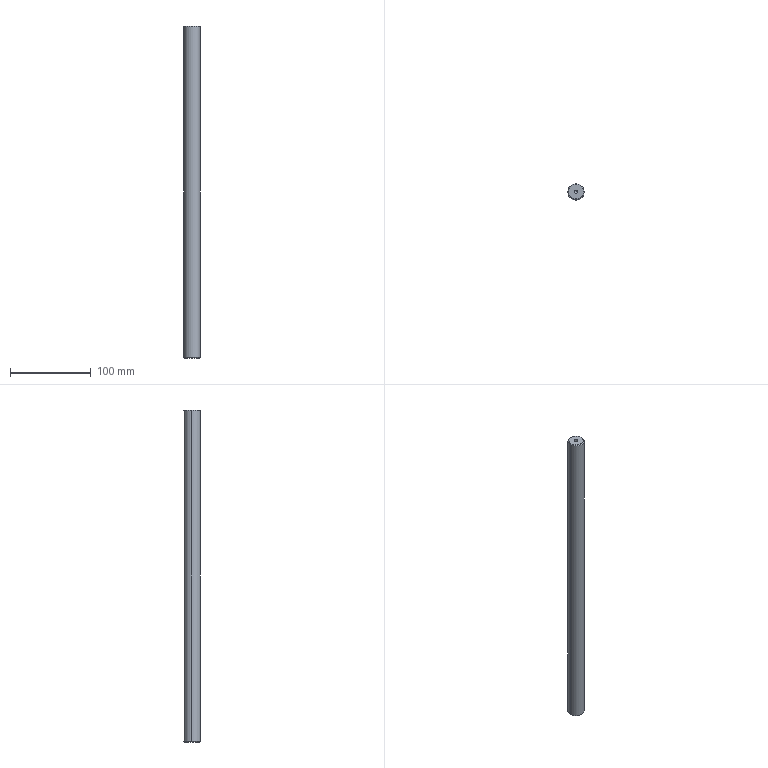Part | STEP file | 1 solid | 12 faces | box 20 x 20 x 410 mm | volume 128595 mm3 | cone 6 | cylinder 4 | plane 2 | commonest cylinder face diameters 4.2 x2 20 x2
STEP:
#1=CARTESIAN_POINT('',(0.,0.,0.));
#2=DIRECTION('',(0.,0.,1.));
#3=DIRECTION('',(1.,0.,0.));
#4=AXIS2_PLACEMENT_3D('',#1,#2,#3);
#5=CARTESIAN_POINT('',(2.1,0.,399.6));
#6=VERTEX_POINT('',#5);
#7=CARTESIAN_POINT('',(2.1,0.,410.));
#8=VERTEX_POINT('',#7);
#9=CARTESIAN_POINT('',(2.1,0.,410.));
#10=DIRECTION('',(0.,0.,1.));
#11=VECTOR('',#10,1.);
#12=LINE('',#9,#11);
#13=CARTESIAN_POINT('',(0.,0.,410.));
#14=DIRECTION('',(0.,0.,1.));
#15=DIRECTION('',(1.,0.,0.));
#16=AXIS2_PLACEMENT_3D('',#13,#14,#15);
#17=CYLINDRICAL_SURFACE('',#16,2.1);
#18=CARTESIAN_POINT('',(6.283,0.));
#19=DIRECTION('',(0.,1.));
#20=VECTOR('',#19,1.);
#21=LINE('',#18,#20);
#22=(GEOMETRIC_REPRESENTATION_CONTEXT(2)PARAMETRIC_REPRESENTATION_CONTEXT()REPRESENTATION_CONTEXT('',''));
#23=DEFINITIONAL_REPRESENTATION('',(#21),#22);
#24=PCURVE('',#17,#23);
#25=CARTESIAN_POINT('',(0.,0.,410.));
#26=DIRECTION('',(0.,0.,1.));
#27=DIRECTION('',(1.,0.,0.));
#28=AXIS2_PLACEMENT_3D('',#25,#26,#27);
#29=CYLINDRICAL_SURFACE('',#28,2.1);
#30=CARTESIAN_POINT('',(0.,0.));
#31=DIRECTION('',(0.,1.));
#32=VECTOR('',#31,1.);
#33=LINE('',#30,#32);
#34=(GEOMETRIC_REPRESENTATION_CONTEXT(2)PARAMETRIC_REPRESENTATION_CONTEXT()REPRESENTATION_CONTEXT('',''));
#35=DEFINITIONAL_REPRESENTATION('',(#33),#34);
#36=PCURVE('',#29,#35);
#37=SURFACE_CURVE('',#12,(#24,#36),.PCURVE_S1.);
#38=EDGE_CURVE('',#6,#8,#37,.T.);
#39=ORIENTED_EDGE('',*,*,#38,.T.);
#40=CARTESIAN_POINT('',(-2.1,0.,410.));
#41=VERTEX_POINT('',#40);
#42=CARTESIAN_POINT('',(0.,0.,410.));
#43=DIRECTION('',(0.,0.,1.));
#44=DIRECTION('',(1.,0.,0.));
#45=AXIS2_PLACEMENT_3D('',#42,#43,#44);
#46=CIRCLE('',#45,2.1);
#47=CARTESIAN_POINT('',(0.,0.));
#48=DIRECTION('',(1.,0.));
#49=VECTOR('',#48,1.);
#50=LINE('',#47,#49);
#51=(GEOMETRIC_REPRESENTATION_CONTEXT(2)PARAMETRIC_REPRESENTATION_CONTEXT()REPRESENTATION_CONTEXT('',''));
#52=DEFINITIONAL_REPRESENTATION('',(#50),#51);
#53=PCURVE('',#17,#52);
#54=CARTESIAN_POINT('',(0.,0.,410.));
#55=DIRECTION('',(0.,0.,1.));
#56=DIRECTION('',(1.,0.,0.));
#57=AXIS2_PLACEMENT_3D('',#54,#55,#56);
#58=PLANE('',#57);
#59=CARTESIAN_POINT('',(0.,0.));
#60=DIRECTION('',(1.,0.));
#61=AXIS2_PLACEMENT_2D('',#59,#60);
#62=CIRCLE('',#61,2.1);
#63=(GEOMETRIC_REPRESENTATION_CONTEXT(2)PARAMETRIC_REPRESENTATION_CONTEXT()REPRESENTATION_CONTEXT('',''));
#64=DEFINITIONAL_REPRESENTATION('',(#62),#63);
#65=PCURVE('',#58,#64);
#66=SURFACE_CURVE('',#46,(#53,#65),.PCURVE_S1.);
#67=EDGE_CURVE('',#41,#8,#66,.T.);
#68=ORIENTED_EDGE('',*,*,#67,.F.);
#69=CARTESIAN_POINT('',(-2.1,0.,399.6));
#70=VERTEX_POINT('',#69);
#71=CARTESIAN_POINT('',(-2.1,0.,410.));
#72=DIRECTION('',(0.,0.,1.));
#73=VECTOR('',#72,1.);
#74=LINE('',#71,#73);
#75=CARTESIAN_POINT('',(3.142,0.));
#76=DIRECTION('',(0.,1.));
#77=VECTOR('',#76,1.);
#78=LINE('',#75,#77);
#79=(GEOMETRIC_REPRESENTATION_CONTEXT(2)PARAMETRIC_REPRESENTATION_CONTEXT()REPRESENTATION_CONTEXT('',''));
#80=DEFINITIONAL_REPRESENTATION('',(#78),#79);
#81=PCURVE('',#17,#80);
#82=CARTESIAN_POINT('',(3.142,0.));
#83=DIRECTION('',(0.,1.));
#84=VECTOR('',#83,1.);
#85=LINE('',#82,#84);
#86=(GEOMETRIC_REPRESENTATION_CONTEXT(2)PARAMETRIC_REPRESENTATION_CONTEXT()REPRESENTATION_CONTEXT('',''));
#87=DEFINITIONAL_REPRESENTATION('',(#85),#86);
#88=PCURVE('',#29,#87);
#89=SURFACE_CURVE('',#74,(#81,#88),.PCURVE_S1.);
#90=EDGE_CURVE('',#70,#41,#89,.T.);
#91=ORIENTED_EDGE('',*,*,#90,.F.);
#92=CARTESIAN_POINT('',(0.,0.,399.6));
#93=DIRECTION('',(0.,0.,1.));
#94=DIRECTION('',(1.,0.,0.));
#95=AXIS2_PLACEMENT_3D('',#92,#93,#94);
#96=CIRCLE('',#95,2.1);
#97=CARTESIAN_POINT('',(0.,-10.4));
#98=DIRECTION('',(1.,0.));
#99=VECTOR('',#98,1.);
#100=LINE('',#97,#99);
#101=(GEOMETRIC_REPRESENTATION_CONTEXT(2)PARAMETRIC_REPRESENTATION_CONTEXT()REPRESENTATION_CONTEXT('',''));
#102=DEFINITIONAL_REPRESENTATION('',(#100),#101);
#103=PCURVE('',#17,#102);
#104=CARTESIAN_POINT('',(0.,0.,399.6));
#105=DIRECTION('',(0.,0.,1.));
#106=DIRECTION('',(1.,0.,0.));
#107=AXIS2_PLACEMENT_3D('',#104,#105,#106);
#108=CONICAL_SURFACE('',#107,2.1,1.03);
#109=CARTESIAN_POINT('',(0.,0.));
#110=DIRECTION('',(1.,0.));
#111=VECTOR('',#110,1.);
#112=LINE('',#109,#111);
#113=(GEOMETRIC_REPRESENTATION_CONTEXT(2)PARAMETRIC_REPRESENTATION_CONTEXT()REPRESENTATION_CONTEXT('',''));
#114=DEFINITIONAL_REPRESENTATION('',(#112),#113);
#115=PCURVE('',#108,#114);
#116=SURFACE_CURVE('',#96,(#103,#115),.PCURVE_S1.);
#117=EDGE_CURVE('',#70,#6,#116,.T.);
#118=ORIENTED_EDGE('',*,*,#117,.T.);
#119=EDGE_LOOP('',(#39,#68,#91,#118));
#120=FACE_BOUND('',#119,.F.);
#121=ADVANCED_FACE('',(#120),#17,.F.);
#122=ORIENTED_EDGE('',*,*,#117,.F.);
#123=CARTESIAN_POINT('',(0.,0.,398.338));
#124=VERTEX_POINT('',#123);
#125=CARTESIAN_POINT('',(-2.1,0.,399.6));
#126=DIRECTION('',(-0.8572,0.,0.515));
#127=VECTOR('',#126,1.);
#128=LINE('',#125,#127);
#129=CARTESIAN_POINT('',(3.142,0.));
#130=DIRECTION('',(0.,1.));
#131=VECTOR('',#130,1.);
#132=LINE('',#129,#131);
#133=(GEOMETRIC_REPRESENTATION_CONTEXT(2)PARAMETRIC_REPRESENTATION_CONTEXT()REPRESENTATION_CONTEXT('',''));
#134=DEFINITIONAL_REPRESENTATION('',(#132),#133);
#135=PCURVE('',#108,#134);
#136=CARTESIAN_POINT('',(0.,0.,399.6));
#137=DIRECTION('',(0.,0.,1.));
#138=DIRECTION('',(1.,0.,0.));
#139=AXIS2_PLACEMENT_3D('',#136,#137,#138);
#140=CONICAL_SURFACE('',#139,2.1,1.03);
#141=CARTESIAN_POINT('',(3.142,0.));
#142=DIRECTION('',(0.,1.));
#143=VECTOR('',#142,1.);
#144=LINE('',#141,#143);
#145=(GEOMETRIC_REPRESENTATION_CONTEXT(2)PARAMETRIC_REPRESENTATION_CONTEXT()REPRESENTATION_CONTEXT('',''));
#146=DEFINITIONAL_REPRESENTATION('',(#144),#145);
#147=PCURVE('',#140,#146);
#148=SURFACE_CURVE('',#128,(#135,#147),.PCURVE_S1.);
#149=EDGE_CURVE('',#124,#70,#148,.T.);
#150=ORIENTED_EDGE('',*,*,#149,.F.);
#151=CARTESIAN_POINT('',(2.1,0.,399.6));
#152=DIRECTION('',(0.8572,0.,0.515));
#153=VECTOR('',#152,1.);
#154=LINE('',#151,#153);
#155=CARTESIAN_POINT('',(6.283,0.));
#156=DIRECTION('',(0.,1.));
#157=VECTOR('',#156,1.);
#158=LINE('',#155,#157);
#159=(GEOMETRIC_REPRESENTATION_CONTEXT(2)PARAMETRIC_REPRESENTATION_CONTEXT()REPRESENTATION_CONTEXT('',''));
#160=DEFINITIONAL_REPRESENTATION('',(#158),#159);
#161=PCURVE('',#108,#160);
#162=CARTESIAN_POINT('',(0.,0.));
#163=DIRECTION('',(0.,1.));
#164=VECTOR('',#163,1.);
#165=LINE('',#162,#164);
#166=(GEOMETRIC_REPRESENTATION_CONTEXT(2)PARAMETRIC_REPRESENTATION_CONTEXT()REPRESENTATION_CONTEXT('',''));
#167=DEFINITIONAL_REPRESENTATION('',(#165),#166);
#168=PCURVE('',#140,#167);
#169=SURFACE_CURVE('',#154,(#161,#168),.PCURVE_S1.);
#170=EDGE_CURVE('',#124,#6,#169,.T.);
#171=ORIENTED_EDGE('',*,*,#170,.T.);
#172=EDGE_LOOP('',(#122,#150,#171));
#173=FACE_BOUND('',#172,.F.);
#174=ADVANCED_FACE('',(#173),#108,.F.);
#175=CARTESIAN_POINT('',(9.,0.,410.));
#176=VERTEX_POINT('',#175);
#177=CARTESIAN_POINT('',(-9.,0.,410.));
#178=VERTEX_POINT('',#177);
#179=CARTESIAN_POINT('',(0.,0.,410.));
#180=DIRECTION('',(0.,0.,1.));
#181=DIRECTION('',(1.,0.,0.));
#182=AXIS2_PLACEMENT_3D('',#179,#180,#181);
#183=CIRCLE('',#182,9.);
#184=CARTESIAN_POINT('',(0.,0.,410.));
#185=DIRECTION('',(0.,0.,-1.));
#186=DIRECTION('',(-1.,0.,0.));
#187=AXIS2_PLACEMENT_3D('',#184,#185,#186);
#188=CONICAL_SURFACE('',#187,9.,0.7854);
#189=CARTESIAN_POINT('',(3.142,0.));
#190=DIRECTION('',(-1.,0.));
#191=VECTOR('',#190,1.);
#192=LINE('',#189,#191);
#193=(GEOMETRIC_REPRESENTATION_CONTEXT(2)PARAMETRIC_REPRESENTATION_CONTEXT()REPRESENTATION_CONTEXT('',''));
#194=DEFINITIONAL_REPRESENTATION('',(#192),#193);
#195=PCURVE('',#188,#194);
#196=CARTESIAN_POINT('',(0.,0.));
#197=DIRECTION('',(1.,0.));
#198=AXIS2_PLACEMENT_2D('',#196,#197);
#199=CIRCLE('',#198,9.);
#200=(GEOMETRIC_REPRESENTATION_CONTEXT(2)PARAMETRIC_REPRESENTATION_CONTEXT()REPRESENTATION_CONTEXT('',''));
#201=DEFINITIONAL_REPRESENTATION('',(#199),#200);
#202=PCURVE('',#58,#201);
#203=SURFACE_CURVE('',#183,(#195,#202),.PCURVE_S1.);
#204=EDGE_CURVE('',#176,#178,#203,.T.);
#205=ORIENTED_EDGE('',*,*,#204,.F.);
#206=CARTESIAN_POINT('',(10.,0.,409.));
#207=VERTEX_POINT('',#206);
#208=CARTESIAN_POINT('',(9.,0.,410.));
#209=DIRECTION('',(0.7071,0.,-0.7071));
#210=VECTOR('',#209,1.);
#211=LINE('',#208,#210);
#212=CARTESIAN_POINT('',(3.142,0.));
#213=DIRECTION('',(0.,1.));
#214=VECTOR('',#213,1.);
#215=LINE('',#212,#214);
#216=(GEOMETRIC_REPRESENTATION_CONTEXT(2)PARAMETRIC_REPRESENTATION_CONTEXT()REPRESENTATION_CONTEXT('',''));
#217=DEFINITIONAL_REPRESENTATION('',(#215),#216);
#218=PCURVE('',#188,#217);
#219=CARTESIAN_POINT('',(0.,0.,410.));
#220=DIRECTION('',(0.,0.,-1.));
#221=DIRECTION('',(-1.,0.,0.));
#222=AXIS2_PLACEMENT_3D('',#219,#220,#221);
#223=CONICAL_SURFACE('',#222,9.,0.7854);
#224=CARTESIAN_POINT('',(3.142,0.));
#225=DIRECTION('',(0.,1.));
#226=VECTOR('',#225,1.);
#227=LINE('',#224,#226);
#228=(GEOMETRIC_REPRESENTATION_CONTEXT(2)PARAMETRIC_REPRESENTATION_CONTEXT()REPRESENTATION_CONTEXT('',''));
#229=DEFINITIONAL_REPRESENTATION('',(#227),#228);
#230=PCURVE('',#223,#229);
#231=SURFACE_CURVE('',#211,(#218,#230),.PCURVE_S1.);
#232=EDGE_CURVE('',#176,#207,#231,.T.);
#233=ORIENTED_EDGE('',*,*,#232,.T.);
#234=CARTESIAN_POINT('',(-10.,0.,409.));
#235=VERTEX_POINT('',#234);
#236=CARTESIAN_POINT('',(0.,0.,409.));
#237=DIRECTION('',(0.,0.,-1.));
#238=DIRECTION('',(1.,0.,0.));
#239=AXIS2_PLACEMENT_3D('',#236,#237,#238);
#240=CIRCLE('',#239,10.);
#241=CARTESIAN_POINT('',(-3.142,1.));
#242=DIRECTION('',(1.,0.));
#243=VECTOR('',#242,1.);
#244=LINE('',#241,#243);
#245=(GEOMETRIC_REPRESENTATION_CONTEXT(2)PARAMETRIC_REPRESENTATION_CONTEXT()REPRESENTATION_CONTEXT('',''));
#246=DEFINITIONAL_REPRESENTATION('',(#244),#245);
#247=PCURVE('',#188,#246);
#248=CARTESIAN_POINT('',(0.,0.,410.));
#249=DIRECTION('',(0.,0.,-1.));
#250=DIRECTION('',(-1.,0.,0.));
#251=AXIS2_PLACEMENT_3D('',#248,#249,#250);
#252=CYLINDRICAL_SURFACE('',#251,10.);
#253=CARTESIAN_POINT('',(-3.142,1.));
#254=DIRECTION('',(1.,0.));
#255=VECTOR('',#254,1.);
#256=LINE('',#253,#255);
#257=(GEOMETRIC_REPRESENTATION_CONTEXT(2)PARAMETRIC_REPRESENTATION_CONTEXT()REPRESENTATION_CONTEXT('',''));
#258=DEFINITIONAL_REPRESENTATION('',(#256),#257);
#259=PCURVE('',#252,#258);
#260=SURFACE_CURVE('',#240,(#247,#259),.PCURVE_S1.);
#261=EDGE_CURVE('',#235,#207,#260,.T.);
#262=ORIENTED_EDGE('',*,*,#261,.F.);
#263=CARTESIAN_POINT('',(-9.,0.,410.));
#264=DIRECTION('',(-0.7071,0.,-0.7071));
#265=VECTOR('',#264,1.);
#266=LINE('',#263,#265);
#267=CARTESIAN_POINT('',(0.,0.));
#268=DIRECTION('',(0.,1.));
#269=VECTOR('',#268,1.);
#270=LINE('',#267,#269);
#271=(GEOMETRIC_REPRESENTATION_CONTEXT(2)PARAMETRIC_REPRESENTATION_CONTEXT()REPRESENTATION_CONTEXT('',''));
#272=DEFINITIONAL_REPRESENTATION('',(#270),#271);
#273=PCURVE('',#188,#272);
#274=CARTESIAN_POINT('',(6.283,0.));
#275=DIRECTION('',(0.,1.));
#276=VECTOR('',#275,1.);
#277=LINE('',#274,#276);
#278=(GEOMETRIC_REPRESENTATION_CONTEXT(2)PARAMETRIC_REPRESENTATION_CONTEXT()REPRESENTATION_CONTEXT('',''));
#279=DEFINITIONAL_REPRESENTATION('',(#277),#278);
#280=PCURVE('',#223,#279);
#281=SURFACE_CURVE('',#266,(#273,#280),.PCURVE_S1.);
#282=EDGE_CURVE('',#178,#235,#281,.T.);
#283=ORIENTED_EDGE('',*,*,#282,.F.);
#284=EDGE_LOOP('',(#205,#233,#262,#283));
#285=FACE_BOUND('',#284,.T.);
#286=ADVANCED_FACE('',(#285),#188,.T.);
#287=CARTESIAN_POINT('',(-9.,0.,0.));
#288=VERTEX_POINT('',#287);
#289=CARTESIAN_POINT('',(9.,0.,0.));
#290=VERTEX_POINT('',#289);
#291=CARTESIAN_POINT('',(0.,0.,0.));
#292=DIRECTION('',(0.,0.,-1.));
#293=DIRECTION('',(1.,0.,0.));
#294=AXIS2_PLACEMENT_3D('',#291,#292,#293);
#295=CIRCLE('',#294,9.);
#296=CARTESIAN_POINT('',(0.,0.,1.));
#297=DIRECTION('',(0.,0.,1.));
#298=DIRECTION('',(1.,0.,0.));
#299=AXIS2_PLACEMENT_3D('',#296,#297,#298);
#300=CONICAL_SURFACE('',#299,10.,0.7854);
#301=CARTESIAN_POINT('',(6.283,-1.));
#302=DIRECTION('',(-1.,0.));
#303=VECTOR('',#302,1.);
#304=LINE('',#301,#303);
#305=(GEOMETRIC_REPRESENTATION_CONTEXT(2)PARAMETRIC_REPRESENTATION_CONTEXT()REPRESENTATION_CONTEXT('',''));
#306=DEFINITIONAL_REPRESENTATION('',(#304),#305);
#307=PCURVE('',#300,#306);
#308=CARTESIAN_POINT('',(0.,0.,0.));
#309=DIRECTION('',(0.,0.,1.));
#310=DIRECTION('',(1.,0.,0.));
#311=AXIS2_PLACEMENT_3D('',#308,#309,#310);
#312=PLANE('',#311);
#313=CARTESIAN_POINT('',(9.,0.));
#314=CARTESIAN_POINT('',(9.,-15.588));
#315=CARTESIAN_POINT('',(-4.5,-7.794));
#316=CARTESIAN_POINT('',(-18.,0.));
#317=CARTESIAN_POINT('',(-4.5,7.794));
#318=CARTESIAN_POINT('',(9.,15.588));
#319=CARTESIAN_POINT('',(9.,0.));
#320=(BOUNDED_CURVE()B_SPLINE_CURVE(2,(#313,#314,#315,#316,#317,#318,#319),.UNSPECIFIED.,.T.,.F.)B_SPLINE_CURVE_WITH_KNOTS((1,2,2,2,2,1),(-2.094,0.,2.094,4.189,6.283,8.378),.UNSPECIFIED.)CURVE()GEOMETRIC_REPRESENTATION_ITEM()RATIONAL_B_SPLINE_CURVE((1.,0.5,1.,0.5,1.,0.5,1.))REPRESENTATION_ITEM(''));
#321=(GEOMETRIC_REPRESENTATION_CONTEXT(2)PARAMETRIC_REPRESENTATION_CONTEXT()REPRESENTATION_CONTEXT('',''));
#322=DEFINITIONAL_REPRESENTATION('',(#320),#321);
#323=PCURVE('',#312,#322);
#324=SURFACE_CURVE('',#295,(#307,#323),.PCURVE_S1.);
#325=EDGE_CURVE('',#288,#290,#324,.T.);
#326=ORIENTED_EDGE('',*,*,#325,.F.);
#327=CARTESIAN_POINT('',(-10.,0.,1.));
#328=VERTEX_POINT('',#327);
#329=CARTESIAN_POINT('',(-10.,0.,1.));
#330=DIRECTION('',(-0.7071,0.,0.7071));
#331=VECTOR('',#330,1.);
#332=LINE('',#329,#331);
#333=CARTESIAN_POINT('',(3.142,0.));
#334=DIRECTION('',(0.,1.));
#335=VECTOR('',#334,1.);
#336=LINE('',#333,#335);
#337=(GEOMETRIC_REPRESENTATION_CONTEXT(2)PARAMETRIC_REPRESENTATION_CONTEXT()REPRESENTATION_CONTEXT('',''));
#338=DEFINITIONAL_REPRESENTATION('',(#336),#337);
#339=PCURVE('',#300,#338);
#340=CARTESIAN_POINT('',(0.,0.,1.));
#341=DIRECTION('',(0.,0.,1.));
#342=DIRECTION('',(1.,0.,0.));
#343=AXIS2_PLACEMENT_3D('',#340,#341,#342);
#344=CONICAL_SURFACE('',#343,10.,0.7854);
#345=CARTESIAN_POINT('',(3.142,0.));
#346=DIRECTION('',(0.,1.));
#347=VECTOR('',#346,1.);
#348=LINE('',#345,#347);
#349=(GEOMETRIC_REPRESENTATION_CONTEXT(2)PARAMETRIC_REPRESENTATION_CONTEXT()REPRESENTATION_CONTEXT('',''));
#350=DEFINITIONAL_REPRESENTATION('',(#348),#349);
#351=PCURVE('',#344,#350);
#352=SURFACE_CURVE('',#332,(#339,#351),.PCURVE_S1.);
#353=EDGE_CURVE('',#288,#328,#352,.T.);
#354=ORIENTED_EDGE('',*,*,#353,.T.);
#355=CARTESIAN_POINT('',(10.,0.,1.));
#356=VERTEX_POINT('',#355);
#357=CARTESIAN_POINT('',(0.,0.,1.));
#358=DIRECTION('',(0.,0.,1.));
#359=DIRECTION('',(1.,0.,0.));
#360=AXIS2_PLACEMENT_3D('',#357,#358,#359);
#361=CIRCLE('',#360,10.);
#362=CARTESIAN_POINT('',(0.,0.));
#363=DIRECTION('',(1.,0.));
#364=VECTOR('',#363,1.);
#365=LINE('',#362,#364);
#366=(GEOMETRIC_REPRESENTATION_CONTEXT(2)PARAMETRIC_REPRESENTATION_CONTEXT()REPRESENTATION_CONTEXT('',''));
#367=DEFINITIONAL_REPRESENTATION('',(#365),#366);
#368=PCURVE('',#300,#367);
#369=CARTESIAN_POINT('',(3.142,409.));
#370=DIRECTION('',(-1.,0.));
#371=VECTOR('',#370,1.);
#372=LINE('',#369,#371);
#373=(GEOMETRIC_REPRESENTATION_CONTEXT(2)PARAMETRIC_REPRESENTATION_CONTEXT()REPRESENTATION_CONTEXT('',''));
#374=DEFINITIONAL_REPRESENTATION('',(#372),#373);
#375=PCURVE('',#252,#374);
#376=SURFACE_CURVE('',#361,(#368,#375),.PCURVE_S1.);
#377=EDGE_CURVE('',#356,#328,#376,.T.);
#378=ORIENTED_EDGE('',*,*,#377,.F.);
#379=CARTESIAN_POINT('',(10.,0.,1.));
#380=DIRECTION('',(0.7071,0.,0.7071));
#381=VECTOR('',#380,1.);
#382=LINE('',#379,#381);
#383=CARTESIAN_POINT('',(0.,0.));
#384=DIRECTION('',(0.,1.));
#385=VECTOR('',#384,1.);
#386=LINE('',#383,#385);
#387=(GEOMETRIC_REPRESENTATION_CONTEXT(2)PARAMETRIC_REPRESENTATION_CONTEXT()REPRESENTATION_CONTEXT('',''));
#388=DEFINITIONAL_REPRESENTATION('',(#386),#387);
#389=PCURVE('',#300,#388);
#390=CARTESIAN_POINT('',(6.283,0.));
#391=DIRECTION('',(0.,1.));
#392=VECTOR('',#391,1.);
#393=LINE('',#390,#392);
#394=(GEOMETRIC_REPRESENTATION_CONTEXT(2)PARAMETRIC_REPRESENTATION_CONTEXT()REPRESENTATION_CONTEXT('',''));
#395=DEFINITIONAL_REPRESENTATION('',(#393),#394);
#396=PCURVE('',#344,#395);
#397=SURFACE_CURVE('',#382,(#389,#396),.PCURVE_S1.);
#398=EDGE_CURVE('',#290,#356,#397,.T.);
#399=ORIENTED_EDGE('',*,*,#398,.F.);
#400=EDGE_LOOP('',(#326,#354,#378,#399));
#401=FACE_BOUND('',#400,.T.);
#402=ADVANCED_FACE('',(#401),#300,.T.);
#403=ORIENTED_EDGE('',*,*,#261,.T.);
#404=CARTESIAN_POINT('',(10.,0.,410.));
#405=DIRECTION('',(0.,0.,-1.));
#406=VECTOR('',#405,1.);
#407=LINE('',#404,#406);
#408=CARTESIAN_POINT('',(3.142,0.));
#409=DIRECTION('',(0.,1.));
#410=VECTOR('',#409,1.);
#411=LINE('',#408,#410);
#412=(GEOMETRIC_REPRESENTATION_CONTEXT(2)PARAMETRIC_REPRESENTATION_CONTEXT()REPRESENTATION_CONTEXT('',''));
#413=DEFINITIONAL_REPRESENTATION('',(#411),#412);
#414=PCURVE('',#252,#413);
#415=CARTESIAN_POINT('',(0.,0.,410.));
#416=DIRECTION('',(0.,0.,-1.));
#417=DIRECTION('',(-1.,0.,0.));
#418=AXIS2_PLACEMENT_3D('',#415,#416,#417);
#419=CYLINDRICAL_SURFACE('',#418,10.);
#420=CARTESIAN_POINT('',(3.142,0.));
#421=DIRECTION('',(0.,1.));
#422=VECTOR('',#421,1.);
#423=LINE('',#420,#422);
#424=(GEOMETRIC_REPRESENTATION_CONTEXT(2)PARAMETRIC_REPRESENTATION_CONTEXT()REPRESENTATION_CONTEXT('',''));
#425=DEFINITIONAL_REPRESENTATION('',(#423),#424);
#426=PCURVE('',#419,#425);
#427=SURFACE_CURVE('',#407,(#414,#426),.PCURVE_S1.);
#428=EDGE_CURVE('',#207,#356,#427,.T.);
#429=ORIENTED_EDGE('',*,*,#428,.T.);
#430=ORIENTED_EDGE('',*,*,#377,.T.);
#431=CARTESIAN_POINT('',(-10.,0.,410.));
#432=DIRECTION('',(0.,0.,-1.));
#433=VECTOR('',#432,1.);
#434=LINE('',#431,#433);
#435=CARTESIAN_POINT('',(0.,0.));
#436=DIRECTION('',(0.,1.));
#437=VECTOR('',#436,1.);
#438=LINE('',#435,#437);
#439=(GEOMETRIC_REPRESENTATION_CONTEXT(2)PARAMETRIC_REPRESENTATION_CONTEXT()REPRESENTATION_CONTEXT('',''));
#440=DEFINITIONAL_REPRESENTATION('',(#438),#439);
#441=PCURVE('',#252,#440);
#442=CARTESIAN_POINT('',(6.283,0.));
#443=DIRECTION('',(0.,1.));
#444=VECTOR('',#443,1.);
#445=LINE('',#442,#444);
#446=(GEOMETRIC_REPRESENTATION_CONTEXT(2)PARAMETRIC_REPRESENTATION_CONTEXT()REPRESENTATION_CONTEXT('',''));
#447=DEFINITIONAL_REPRESENTATION('',(#445),#446);
#448=PCURVE('',#419,#447);
#449=SURFACE_CURVE('',#434,(#441,#448),.PCURVE_S1.);
#450=EDGE_CURVE('',#235,#328,#449,.T.);
#451=ORIENTED_EDGE('',*,*,#450,.F.);
#452=EDGE_LOOP('',(#403,#429,#430,#451));
#453=FACE_BOUND('',#452,.T.);
#454=ADVANCED_FACE('',(#453),#252,.T.);
#455=ORIENTED_EDGE('',*,*,#428,.F.);
#456=CARTESIAN_POINT('',(0.,0.,409.));
#457=DIRECTION('',(0.,0.,-1.));
#458=DIRECTION('',(1.,0.,0.));
#459=AXIS2_PLACEMENT_3D('',#456,#457,#458);
#460=CIRCLE('',#459,10.);
#461=CARTESIAN_POINT('',(3.142,1.));
#462=DIRECTION('',(1.,0.));
#463=VECTOR('',#462,1.);
#464=LINE('',#461,#463);
#465=(GEOMETRIC_REPRESENTATION_CONTEXT(2)PARAMETRIC_REPRESENTATION_CONTEXT()REPRESENTATION_CONTEXT('',''));
#466=DEFINITIONAL_REPRESENTATION('',(#464),#465);
#467=PCURVE('',#419,#466);
#468=CARTESIAN_POINT('',(3.142,1.));
#469=DIRECTION('',(1.,0.));
#470=VECTOR('',#469,1.);
#471=LINE('',#468,#470);
#472=(GEOMETRIC_REPRESENTATION_CONTEXT(2)PARAMETRIC_REPRESENTATION_CONTEXT()REPRESENTATION_CONTEXT('',''));
#473=DEFINITIONAL_REPRESENTATION('',(#471),#472);
#474=PCURVE('',#223,#473);
#475=SURFACE_CURVE('',#460,(#467,#474),.PCURVE_S1.);
#476=EDGE_CURVE('',#207,#235,#475,.T.);
#477=ORIENTED_EDGE('',*,*,#476,.T.);
#478=ORIENTED_EDGE('',*,*,#450,.T.);
#479=CARTESIAN_POINT('',(0.,0.,1.));
#480=DIRECTION('',(0.,0.,1.));
#481=DIRECTION('',(1.,0.,0.));
#482=AXIS2_PLACEMENT_3D('',#479,#480,#481);
#483=CIRCLE('',#482,10.);
#484=CARTESIAN_POINT('',(9.425,409.));
#485=DIRECTION('',(-1.,0.));
#486=VECTOR('',#485,1.);
#487=LINE('',#484,#486);
#488=(GEOMETRIC_REPRESENTATION_CONTEXT(2)PARAMETRIC_REPRESENTATION_CONTEXT()REPRESENTATION_CONTEXT('',''));
#489=DEFINITIONAL_REPRESENTATION('',(#487),#488);
#490=PCURVE('',#419,#489);
#491=CARTESIAN_POINT('',(0.,0.));
#492=DIRECTION('',(1.,0.));
#493=VECTOR('',#492,1.);
#494=LINE('',#491,#493);
#495=(GEOMETRIC_REPRESENTATION_CONTEXT(2)PARAMETRIC_REPRESENTATION_CONTEXT()REPRESENTATION_CONTEXT('',''));
#496=DEFINITIONAL_REPRESENTATION('',(#494),#495);
#497=PCURVE('',#344,#496);
#498=SURFACE_CURVE('',#483,(#490,#497),.PCURVE_S1.);
#499=EDGE_CURVE('',#328,#356,#498,.T.);
#500=ORIENTED_EDGE('',*,*,#499,.T.);
#501=EDGE_LOOP('',(#455,#477,#478,#500));
#502=FACE_BOUND('',#501,.T.);
#503=ADVANCED_FACE('',(#502),#419,.T.);
#504=CARTESIAN_POINT('',(0.,0.,410.));
#505=DIRECTION('',(0.,0.,1.));
#506=DIRECTION('',(1.,0.,0.));
#507=AXIS2_PLACEMENT_3D('',#504,#505,#506);
#508=CIRCLE('',#507,2.1);
#509=CARTESIAN_POINT('',(0.,0.));
#510=DIRECTION('',(1.,0.));
#511=AXIS2_PLACEMENT_2D('',#509,#510);
#512=CIRCLE('',#511,2.1);
#513=(GEOMETRIC_REPRESENTATION_CONTEXT(2)PARAMETRIC_REPRESENTATION_CONTEXT()REPRESENTATION_CONTEXT('',''));
#514=DEFINITIONAL_REPRESENTATION('',(#512),#513);
#515=PCURVE('',#58,#514);
#516=CARTESIAN_POINT('',(0.,0.));
#517=DIRECTION('',(1.,0.));
#518=VECTOR('',#517,1.);
#519=LINE('',#516,#518);
#520=(GEOMETRIC_REPRESENTATION_CONTEXT(2)PARAMETRIC_REPRESENTATION_CONTEXT()REPRESENTATION_CONTEXT('',''));
#521=DEFINITIONAL_REPRESENTATION('',(#519),#520);
#522=PCURVE('',#29,#521);
#523=SURFACE_CURVE('',#508,(#515,#522),.PCURVE_S1.);
#524=EDGE_CURVE('',#8,#41,#523,.T.);
#525=ORIENTED_EDGE('',*,*,#524,.F.);
#526=ORIENTED_EDGE('',*,*,#67,.F.);
#527=EDGE_LOOP('',(#525,#526));
#528=FACE_BOUND('',#527,.T.);
#529=CARTESIAN_POINT('',(0.,0.,410.));
#530=DIRECTION('',(0.,0.,1.));
#531=DIRECTION('',(1.,0.,0.));
#532=AXIS2_PLACEMENT_3D('',#529,#530,#531);
#533=CIRCLE('',#532,9.);
#534=CARTESIAN_POINT('',(0.,0.));
#535=DIRECTION('',(1.,0.));
#536=AXIS2_PLACEMENT_2D('',#534,#535);
#537=CIRCLE('',#536,9.);
#538=(GEOMETRIC_REPRESENTATION_CONTEXT(2)PARAMETRIC_REPRESENTATION_CONTEXT()REPRESENTATION_CONTEXT('',''));
#539=DEFINITIONAL_REPRESENTATION('',(#537),#538);
#540=PCURVE('',#58,#539);
#541=CARTESIAN_POINT('',(9.425,0.));
#542=DIRECTION('',(-1.,0.));
#543=VECTOR('',#542,1.);
#544=LINE('',#541,#543);
#545=(GEOMETRIC_REPRESENTATION_CONTEXT(2)PARAMETRIC_REPRESENTATION_CONTEXT()REPRESENTATION_CONTEXT('',''));
#546=DEFINITIONAL_REPRESENTATION('',(#544),#545);
#547=PCURVE('',#223,#546);
#548=SURFACE_CURVE('',#533,(#540,#547),.PCURVE_S1.);
#549=EDGE_CURVE('',#178,#176,#548,.T.);
#550=ORIENTED_EDGE('',*,*,#549,.T.);
#551=ORIENTED_EDGE('',*,*,#204,.T.);
#552=EDGE_LOOP('',(#550,#551));
#553=FACE_BOUND('',#552,.T.);
#554=ADVANCED_FACE('',(#528,#553),#58,.T.);
#555=CARTESIAN_POINT('',(0.,0.,0.));
#556=DIRECTION('',(0.,0.,-1.));
#557=DIRECTION('',(1.,0.,0.));
#558=AXIS2_PLACEMENT_3D('',#555,#556,#557);
#559=CIRCLE('',#558,9.);
#560=CARTESIAN_POINT('',(9.,0.));
#561=CARTESIAN_POINT('',(9.,-15.588));
#562=CARTESIAN_POINT('',(-4.5,-7.794));
#563=CARTESIAN_POINT('',(-18.,0.));
#564=CARTESIAN_POINT('',(-4.5,7.794));
#565=CARTESIAN_POINT('',(9.,15.588));
#566=CARTESIAN_POINT('',(9.,0.));
#567=(BOUNDED_CURVE()B_SPLINE_CURVE(2,(#560,#561,#562,#563,#564,#565,#566),.UNSPECIFIED.,.T.,.F.)B_SPLINE_CURVE_WITH_KNOTS((1,2,2,2,2,1),(-2.094,0.,2.094,4.189,6.283,8.378),.UNSPECIFIED.)CURVE()GEOMETRIC_REPRESENTATION_ITEM()RATIONAL_B_SPLINE_CURVE((1.,0.5,1.,0.5,1.,0.5,1.))REPRESENTATION_ITEM(''));
#568=(GEOMETRIC_REPRESENTATION_CONTEXT(2)PARAMETRIC_REPRESENTATION_CONTEXT()REPRESENTATION_CONTEXT('',''));
#569=DEFINITIONAL_REPRESENTATION('',(#567),#568);
#570=PCURVE('',#312,#569);
#571=CARTESIAN_POINT('',(6.283,-1.));
#572=DIRECTION('',(-1.,0.));
#573=VECTOR('',#572,1.);
#574=LINE('',#571,#573);
#575=(GEOMETRIC_REPRESENTATION_CONTEXT(2)PARAMETRIC_REPRESENTATION_CONTEXT()REPRESENTATION_CONTEXT('',''));
#576=DEFINITIONAL_REPRESENTATION('',(#574),#575);
#577=PCURVE('',#344,#576);
#578=SURFACE_CURVE('',#559,(#570,#577),.PCURVE_S1.);
#579=EDGE_CURVE('',#290,#288,#578,.T.);
#580=ORIENTED_EDGE('',*,*,#579,.T.);
#581=ORIENTED_EDGE('',*,*,#325,.T.);
#582=EDGE_LOOP('',(#580,#581));
#583=FACE_BOUND('',#582,.T.);
#584=ADVANCED_FACE('',(#583),#312,.F.);
#585=ORIENTED_EDGE('',*,*,#353,.F.);
#586=ORIENTED_EDGE('',*,*,#579,.F.);
#587=ORIENTED_EDGE('',*,*,#398,.T.);
#588=ORIENTED_EDGE('',*,*,#499,.F.);
#589=EDGE_LOOP('',(#585,#586,#587,#588));
#590=FACE_BOUND('',#589,.T.);
#591=ADVANCED_FACE('',(#590),#344,.T.);
#592=ORIENTED_EDGE('',*,*,#232,.F.);
#593=ORIENTED_EDGE('',*,*,#549,.F.);
#594=ORIENTED_EDGE('',*,*,#282,.T.);
#595=ORIENTED_EDGE('',*,*,#476,.F.);
#596=EDGE_LOOP('',(#592,#593,#594,#595));
#597=FACE_BOUND('',#596,.T.);
#598=ADVANCED_FACE('',(#597),#223,.T.);
#599=CARTESIAN_POINT('',(0.,0.,399.6));
#600=DIRECTION('',(0.,0.,1.));
#601=DIRECTION('',(1.,0.,0.));
#602=AXIS2_PLACEMENT_3D('',#599,#600,#601);
#603=CIRCLE('',#602,2.1);
#604=CARTESIAN_POINT('',(0.,0.));
#605=DIRECTION('',(1.,0.));
#606=VECTOR('',#605,1.);
#607=LINE('',#604,#606);
#608=(GEOMETRIC_REPRESENTATION_CONTEXT(2)PARAMETRIC_REPRESENTATION_CONTEXT()REPRESENTATION_CONTEXT('',''));
#609=DEFINITIONAL_REPRESENTATION('',(#607),#608);
#610=PCURVE('',#140,#609);
#611=CARTESIAN_POINT('',(0.,-10.4));
#612=DIRECTION('',(1.,0.));
#613=VECTOR('',#612,1.);
#614=LINE('',#611,#613);
#615=(GEOMETRIC_REPRESENTATION_CONTEXT(2)PARAMETRIC_REPRESENTATION_CONTEXT()REPRESENTATION_CONTEXT('',''));
#616=DEFINITIONAL_REPRESENTATION('',(#614),#615);
#617=PCURVE('',#29,#616);
#618=SURFACE_CURVE('',#603,(#610,#617),.PCURVE_S1.);
#619=EDGE_CURVE('',#6,#70,#618,.T.);
#620=ORIENTED_EDGE('',*,*,#619,.F.);
#621=ORIENTED_EDGE('',*,*,#170,.F.);
#622=ORIENTED_EDGE('',*,*,#149,.T.);
#623=EDGE_LOOP('',(#620,#621,#622));
#624=FACE_BOUND('',#623,.F.);
#625=ADVANCED_FACE('',(#624),#140,.F.);
#626=ORIENTED_EDGE('',*,*,#524,.F.);
#627=ORIENTED_EDGE('',*,*,#38,.F.);
#628=ORIENTED_EDGE('',*,*,#619,.T.);
#629=ORIENTED_EDGE('',*,*,#90,.T.);
#630=EDGE_LOOP('',(#626,#627,#628,#629));
#631=FACE_BOUND('',#630,.F.);
#632=ADVANCED_FACE('',(#631),#29,.F.);
#633=CLOSED_SHELL('',(#121,#174,#286,#402,#454,#503,#554,#584,#591,#598,#625,#632));
#634=MANIFOLD_SOLID_BREP('',#633);
#635=(LENGTH_UNIT()NAMED_UNIT(*)SI_UNIT(.MILLI.,.METRE.));
#636=UNCERTAINTY_MEASURE_WITH_UNIT(LENGTH_MEASURE(0.0000001),#635,'','');
#637=(NAMED_UNIT(*)PLANE_ANGLE_UNIT()SI_UNIT($,.RADIAN.));
#638=(NAMED_UNIT(*)SI_UNIT($,.STERADIAN.)SOLID_ANGLE_UNIT());
#639=(GEOMETRIC_REPRESENTATION_CONTEXT(3)GLOBAL_UNCERTAINTY_ASSIGNED_CONTEXT((#636))GLOBAL_UNIT_ASSIGNED_CONTEXT((#635,#637,#638))REPRESENTATION_CONTEXT('',''));
#640=ADVANCED_BREP_SHAPE_REPRESENTATION('',(#4,#634),#639);